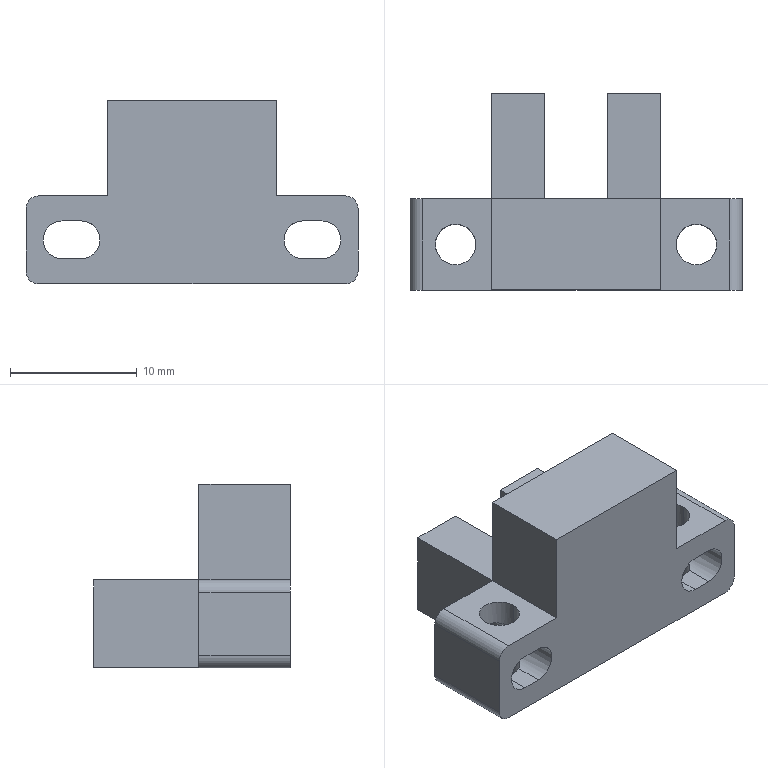Part | SolidWorks | features ICE 3, Extrusion 1, Fillet 1 | 1 solid | 44 faces | box 26.2 x 15.5 x 14.5 mm | volume 2285 mm3 | plane 28 | cylinder 16 | commonest cylinder face diameters 3.2 x8 2 x4 3 x4